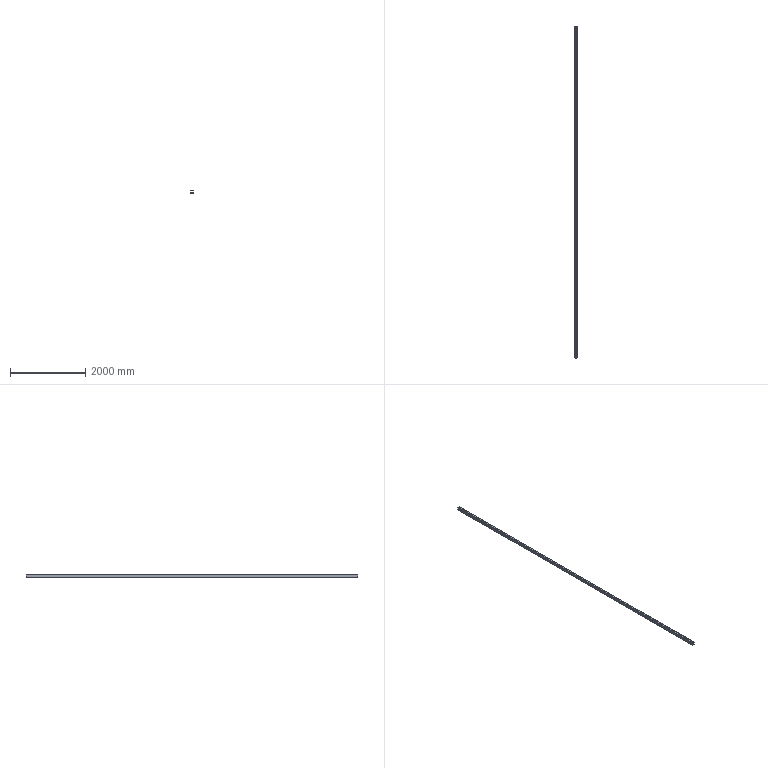Part | SolidWorks | features WeldMemberFeat 1, WeldmentFeature 1 | 1 solid | 18 faces | box 60 x 8850 x 80 mm | volume 10935232 mm3 | plane 10 | cylinder 8 | commonest cylinder face diameters 10 x4 20 x4
STEP:
#1=CARTESIAN_POINT('',(-30.,0.,30.));
#2=VERTEX_POINT('',#1);
#3=CARTESIAN_POINT('',(-20.,0.,40.));
#4=VERTEX_POINT('',#3);
#5=CARTESIAN_POINT('',(-20.,0.,30.));
#6=DIRECTION('',(0.,1.,0.));
#7=DIRECTION('',(0.,0.,1.));
#8=AXIS2_PLACEMENT_3D('',#5,#6,#7);
#9=CIRCLE('',#8,10.);
#10=EDGE_CURVE('',#2,#4,#9,.T.);
#11=ORIENTED_EDGE('',*,*,#10,.T.);
#12=CARTESIAN_POINT('',(-20.,8850.,40.));
#13=VERTEX_POINT('',#12);
#14=CARTESIAN_POINT('',(-20.,8850.,40.));
#15=DIRECTION('',(0.,-1.,0.));
#16=VECTOR('',#15,1000.);
#17=LINE('',#14,#16);
#18=EDGE_CURVE('',#13,#4,#17,.T.);
#19=ORIENTED_EDGE('',*,*,#18,.F.);
#20=CARTESIAN_POINT('',(-30.,8850.,30.));
#21=VERTEX_POINT('',#20);
#22=CARTESIAN_POINT('',(-20.,8850.,30.));
#23=DIRECTION('',(0.,1.,0.));
#24=DIRECTION('',(0.,0.,1.));
#25=AXIS2_PLACEMENT_3D('',#22,#23,#24);
#26=CIRCLE('',#25,10.);
#27=EDGE_CURVE('',#21,#13,#26,.T.);
#28=ORIENTED_EDGE('',*,*,#27,.F.);
#29=CARTESIAN_POINT('',(-30.,8850.,30.));
#30=DIRECTION('',(0.,-1.,0.));
#31=VECTOR('',#30,1000.);
#32=LINE('',#29,#31);
#33=EDGE_CURVE('',#21,#2,#32,.T.);
#34=ORIENTED_EDGE('',*,*,#33,.T.);
#35=EDGE_LOOP('',(#11,#19,#28,#34));
#36=FACE_OUTER_BOUND('',#35,.T.);
#37=CARTESIAN_POINT('',(-20.,8850.,30.));
#38=DIRECTION('',(0.,-1.,0.));
#39=DIRECTION('',(0.,0.,-1.));
#40=AXIS2_PLACEMENT_3D('',#37,#38,#39);
#41=CYLINDRICAL_SURFACE('',#40,10.);
#42=ADVANCED_FACE('',(#36),#41,.T.);
#43=CARTESIAN_POINT('',(20.,0.,40.));
#44=VERTEX_POINT('',#43);
#45=CARTESIAN_POINT('',(-20.,0.,40.));
#46=DIRECTION('',(1.,0.,0.));
#47=VECTOR('',#46,1000.);
#48=LINE('',#45,#47);
#49=EDGE_CURVE('',#4,#44,#48,.T.);
#50=ORIENTED_EDGE('',*,*,#49,.T.);
#51=CARTESIAN_POINT('',(20.,8850.,40.));
#52=VERTEX_POINT('',#51);
#53=CARTESIAN_POINT('',(20.,8850.,40.));
#54=DIRECTION('',(0.,-1.,0.));
#55=VECTOR('',#54,1000.);
#56=LINE('',#53,#55);
#57=EDGE_CURVE('',#52,#44,#56,.T.);
#58=ORIENTED_EDGE('',*,*,#57,.F.);
#59=CARTESIAN_POINT('',(-20.,8850.,40.));
#60=DIRECTION('',(1.,0.,0.));
#61=VECTOR('',#60,1000.);
#62=LINE('',#59,#61);
#63=EDGE_CURVE('',#13,#52,#62,.T.);
#64=ORIENTED_EDGE('',*,*,#63,.F.);
#65=ORIENTED_EDGE('',*,*,#18,.T.);
#66=EDGE_LOOP('',(#50,#58,#64,#65));
#67=FACE_OUTER_BOUND('',#66,.T.);
#68=CARTESIAN_POINT('',(-20.,8850.,40.));
#69=DIRECTION('',(0.,0.,-1.));
#70=DIRECTION('',(-1.,0.,0.));
#71=AXIS2_PLACEMENT_3D('',#68,#69,#70);
#72=PLANE('',#71);
#73=ADVANCED_FACE('',(#67),#72,.F.);
#74=CARTESIAN_POINT('',(30.,0.,30.));
#75=VERTEX_POINT('',#74);
#76=CARTESIAN_POINT('',(20.,0.,30.));
#77=DIRECTION('',(0.,1.,0.));
#78=DIRECTION('',(0.,0.,1.));
#79=AXIS2_PLACEMENT_3D('',#76,#77,#78);
#80=CIRCLE('',#79,10.);
#81=EDGE_CURVE('',#44,#75,#80,.T.);
#82=ORIENTED_EDGE('',*,*,#81,.T.);
#83=CARTESIAN_POINT('',(30.,8850.,30.));
#84=VERTEX_POINT('',#83);
#85=CARTESIAN_POINT('',(30.,8850.,30.));
#86=DIRECTION('',(0.,-1.,0.));
#87=VECTOR('',#86,1000.);
#88=LINE('',#85,#87);
#89=EDGE_CURVE('',#84,#75,#88,.T.);
#90=ORIENTED_EDGE('',*,*,#89,.F.);
#91=CARTESIAN_POINT('',(20.,8850.,30.));
#92=DIRECTION('',(0.,1.,0.));
#93=DIRECTION('',(0.,0.,1.));
#94=AXIS2_PLACEMENT_3D('',#91,#92,#93);
#95=CIRCLE('',#94,10.);
#96=EDGE_CURVE('',#52,#84,#95,.T.);
#97=ORIENTED_EDGE('',*,*,#96,.F.);
#98=ORIENTED_EDGE('',*,*,#57,.T.);
#99=EDGE_LOOP('',(#82,#90,#97,#98));
#100=FACE_OUTER_BOUND('',#99,.T.);
#101=CARTESIAN_POINT('',(20.,8850.,30.));
#102=DIRECTION('',(0.,-1.,0.));
#103=DIRECTION('',(0.,0.,-1.));
#104=AXIS2_PLACEMENT_3D('',#101,#102,#103);
#105=CYLINDRICAL_SURFACE('',#104,10.);
#106=ADVANCED_FACE('',(#100),#105,.T.);
#107=CARTESIAN_POINT('',(30.,0.,-30.));
#108=VERTEX_POINT('',#107);
#109=CARTESIAN_POINT('',(30.,0.,-30.));
#110=DIRECTION('',(0.,0.,-1.));
#111=VECTOR('',#110,1000.);
#112=LINE('',#109,#111);
#113=EDGE_CURVE('',#75,#108,#112,.T.);
#114=ORIENTED_EDGE('',*,*,#113,.T.);
#115=CARTESIAN_POINT('',(30.,8850.,-30.));
#116=VERTEX_POINT('',#115);
#117=CARTESIAN_POINT('',(30.,8850.,-30.));
#118=DIRECTION('',(0.,-1.,0.));
#119=VECTOR('',#118,1000.);
#120=LINE('',#117,#119);
#121=EDGE_CURVE('',#116,#108,#120,.T.);
#122=ORIENTED_EDGE('',*,*,#121,.F.);
#123=CARTESIAN_POINT('',(30.,8850.,-30.));
#124=DIRECTION('',(0.,0.,-1.));
#125=VECTOR('',#124,1000.);
#126=LINE('',#123,#125);
#127=EDGE_CURVE('',#84,#116,#126,.T.);
#128=ORIENTED_EDGE('',*,*,#127,.F.);
#129=ORIENTED_EDGE('',*,*,#89,.T.);
#130=EDGE_LOOP('',(#114,#122,#128,#129));
#131=FACE_OUTER_BOUND('',#130,.T.);
#132=CARTESIAN_POINT('',(30.,8850.,-30.));
#133=DIRECTION('',(-1.,0.,0.));
#134=DIRECTION('',(0.,0.,1.));
#135=AXIS2_PLACEMENT_3D('',#132,#133,#134);
#136=PLANE('',#135);
#137=ADVANCED_FACE('',(#131),#136,.F.);
#138=CARTESIAN_POINT('',(20.,0.,-40.));
#139=VERTEX_POINT('',#138);
#140=CARTESIAN_POINT('',(20.,0.,-30.));
#141=DIRECTION('',(0.,1.,0.));
#142=DIRECTION('',(0.,0.,1.));
#143=AXIS2_PLACEMENT_3D('',#140,#141,#142);
#144=CIRCLE('',#143,10.);
#145=EDGE_CURVE('',#108,#139,#144,.T.);
#146=ORIENTED_EDGE('',*,*,#145,.T.);
#147=CARTESIAN_POINT('',(20.,8850.,-40.));
#148=VERTEX_POINT('',#147);
#149=CARTESIAN_POINT('',(20.,8850.,-40.));
#150=DIRECTION('',(0.,-1.,0.));
#151=VECTOR('',#150,1000.);
#152=LINE('',#149,#151);
#153=EDGE_CURVE('',#148,#139,#152,.T.);
#154=ORIENTED_EDGE('',*,*,#153,.F.);
#155=CARTESIAN_POINT('',(20.,8850.,-30.));
#156=DIRECTION('',(0.,1.,0.));
#157=DIRECTION('',(0.,0.,1.));
#158=AXIS2_PLACEMENT_3D('',#155,#156,#157);
#159=CIRCLE('',#158,10.);
#160=EDGE_CURVE('',#116,#148,#159,.T.);
#161=ORIENTED_EDGE('',*,*,#160,.F.);
#162=ORIENTED_EDGE('',*,*,#121,.T.);
#163=EDGE_LOOP('',(#146,#154,#161,#162));
#164=FACE_OUTER_BOUND('',#163,.T.);
#165=CARTESIAN_POINT('',(20.,8850.,-30.));
#166=DIRECTION('',(0.,-1.,0.));
#167=DIRECTION('',(0.,0.,-1.));
#168=AXIS2_PLACEMENT_3D('',#165,#166,#167);
#169=CYLINDRICAL_SURFACE('',#168,10.);
#170=ADVANCED_FACE('',(#164),#169,.T.);
#171=CARTESIAN_POINT('',(-20.,0.,-40.));
#172=VERTEX_POINT('',#171);
#173=CARTESIAN_POINT('',(20.,0.,-40.));
#174=DIRECTION('',(-1.,0.,0.));
#175=VECTOR('',#174,1000.);
#176=LINE('',#173,#175);
#177=EDGE_CURVE('',#139,#172,#176,.T.);
#178=ORIENTED_EDGE('',*,*,#177,.T.);
#179=CARTESIAN_POINT('',(-20.,8850.,-40.));
#180=VERTEX_POINT('',#179);
#181=CARTESIAN_POINT('',(-20.,8850.,-40.));
#182=DIRECTION('',(0.,-1.,0.));
#183=VECTOR('',#182,1000.);
#184=LINE('',#181,#183);
#185=EDGE_CURVE('',#180,#172,#184,.T.);
#186=ORIENTED_EDGE('',*,*,#185,.F.);
#187=CARTESIAN_POINT('',(20.,8850.,-40.));
#188=DIRECTION('',(-1.,0.,0.));
#189=VECTOR('',#188,1000.);
#190=LINE('',#187,#189);
#191=EDGE_CURVE('',#148,#180,#190,.T.);
#192=ORIENTED_EDGE('',*,*,#191,.F.);
#193=ORIENTED_EDGE('',*,*,#153,.T.);
#194=EDGE_LOOP('',(#178,#186,#192,#193));
#195=FACE_OUTER_BOUND('',#194,.T.);
#196=CARTESIAN_POINT('',(20.,8850.,-40.));
#197=DIRECTION('',(0.,0.,1.));
#198=DIRECTION('',(1.,0.,0.));
#199=AXIS2_PLACEMENT_3D('',#196,#197,#198);
#200=PLANE('',#199);
#201=ADVANCED_FACE('',(#195),#200,.F.);
#202=CARTESIAN_POINT('',(-30.,0.,-30.));
#203=VERTEX_POINT('',#202);
#204=CARTESIAN_POINT('',(-20.,0.,-30.));
#205=DIRECTION('',(0.,1.,0.));
#206=DIRECTION('',(0.,0.,1.));
#207=AXIS2_PLACEMENT_3D('',#204,#205,#206);
#208=CIRCLE('',#207,10.);
#209=EDGE_CURVE('',#172,#203,#208,.T.);
#210=ORIENTED_EDGE('',*,*,#209,.T.);
#211=CARTESIAN_POINT('',(-30.,8850.,-30.));
#212=VERTEX_POINT('',#211);
#213=CARTESIAN_POINT('',(-30.,8850.,-30.));
#214=DIRECTION('',(0.,-1.,0.));
#215=VECTOR('',#214,1000.);
#216=LINE('',#213,#215);
#217=EDGE_CURVE('',#212,#203,#216,.T.);
#218=ORIENTED_EDGE('',*,*,#217,.F.);
#219=CARTESIAN_POINT('',(-20.,8850.,-30.));
#220=DIRECTION('',(0.,1.,0.));
#221=DIRECTION('',(0.,0.,1.));
#222=AXIS2_PLACEMENT_3D('',#219,#220,#221);
#223=CIRCLE('',#222,10.);
#224=EDGE_CURVE('',#180,#212,#223,.T.);
#225=ORIENTED_EDGE('',*,*,#224,.F.);
#226=ORIENTED_EDGE('',*,*,#185,.T.);
#227=EDGE_LOOP('',(#210,#218,#225,#226));
#228=FACE_OUTER_BOUND('',#227,.T.);
#229=CARTESIAN_POINT('',(-20.,8850.,-30.));
#230=DIRECTION('',(0.,-1.,0.));
#231=DIRECTION('',(0.,0.,-1.));
#232=AXIS2_PLACEMENT_3D('',#229,#230,#231);
#233=CYLINDRICAL_SURFACE('',#232,10.);
#234=ADVANCED_FACE('',(#228),#233,.T.);
#235=CARTESIAN_POINT('',(20.,0.,35.));
#236=VERTEX_POINT('',#235);
#237=CARTESIAN_POINT('',(25.,0.,30.));
#238=VERTEX_POINT('',#237);
#239=CARTESIAN_POINT('',(20.,0.,30.));
#240=DIRECTION('',(0.,1.,0.));
#241=DIRECTION('',(0.,0.,1.));
#242=AXIS2_PLACEMENT_3D('',#239,#240,#241);
#243=CIRCLE('',#242,5.);
#244=EDGE_CURVE('',#236,#238,#243,.T.);
#245=ORIENTED_EDGE('',*,*,#244,.F.);
#246=CARTESIAN_POINT('',(20.,8850.,35.));
#247=VERTEX_POINT('',#246);
#248=CARTESIAN_POINT('',(20.,8850.,35.));
#249=DIRECTION('',(0.,-1.,0.));
#250=VECTOR('',#249,1000.);
#251=LINE('',#248,#250);
#252=EDGE_CURVE('',#247,#236,#251,.T.);
#253=ORIENTED_EDGE('',*,*,#252,.F.);
#254=CARTESIAN_POINT('',(25.,8850.,30.));
#255=VERTEX_POINT('',#254);
#256=CARTESIAN_POINT('',(20.,8850.,30.));
#257=DIRECTION('',(0.,1.,0.));
#258=DIRECTION('',(0.,0.,1.));
#259=AXIS2_PLACEMENT_3D('',#256,#257,#258);
#260=CIRCLE('',#259,5.);
#261=EDGE_CURVE('',#247,#255,#260,.T.);
#262=ORIENTED_EDGE('',*,*,#261,.T.);
#263=CARTESIAN_POINT('',(25.,8850.,30.));
#264=DIRECTION('',(0.,-1.,0.));
#265=VECTOR('',#264,1000.);
#266=LINE('',#263,#265);
#267=EDGE_CURVE('',#255,#238,#266,.T.);
#268=ORIENTED_EDGE('',*,*,#267,.T.);
#269=EDGE_LOOP('',(#245,#253,#262,#268));
#270=FACE_OUTER_BOUND('',#269,.T.);
#271=CARTESIAN_POINT('',(20.,8850.,30.));
#272=DIRECTION('',(0.,-1.,0.));
#273=DIRECTION('',(0.,0.,-1.));
#274=AXIS2_PLACEMENT_3D('',#271,#272,#273);
#275=CYLINDRICAL_SURFACE('',#274,5.);
#276=ADVANCED_FACE('',(#270),#275,.F.);
#277=CARTESIAN_POINT('',(-20.,0.,35.));
#278=VERTEX_POINT('',#277);
#279=CARTESIAN_POINT('',(-20.,0.,35.));
#280=DIRECTION('',(1.,0.,0.));
#281=VECTOR('',#280,1000.);
#282=LINE('',#279,#281);
#283=EDGE_CURVE('',#278,#236,#282,.T.);
#284=ORIENTED_EDGE('',*,*,#283,.F.);
#285=CARTESIAN_POINT('',(-20.,8850.,35.));
#286=VERTEX_POINT('',#285);
#287=CARTESIAN_POINT('',(-20.,8850.,35.));
#288=DIRECTION('',(0.,-1.,0.));
#289=VECTOR('',#288,1000.);
#290=LINE('',#287,#289);
#291=EDGE_CURVE('',#286,#278,#290,.T.);
#292=ORIENTED_EDGE('',*,*,#291,.F.);
#293=CARTESIAN_POINT('',(-20.,8850.,35.));
#294=DIRECTION('',(1.,0.,0.));
#295=VECTOR('',#294,1000.);
#296=LINE('',#293,#295);
#297=EDGE_CURVE('',#286,#247,#296,.T.);
#298=ORIENTED_EDGE('',*,*,#297,.T.);
#299=ORIENTED_EDGE('',*,*,#252,.T.);
#300=EDGE_LOOP('',(#284,#292,#298,#299));
#301=FACE_OUTER_BOUND('',#300,.T.);
#302=CARTESIAN_POINT('',(-20.,8850.,35.));
#303=DIRECTION('',(0.,0.,-1.));
#304=DIRECTION('',(-1.,0.,0.));
#305=AXIS2_PLACEMENT_3D('',#302,#303,#304);
#306=PLANE('',#305);
#307=ADVANCED_FACE('',(#301),#306,.T.);
#308=CARTESIAN_POINT('',(-25.,0.,30.));
#309=VERTEX_POINT('',#308);
#310=CARTESIAN_POINT('',(-20.,0.,30.));
#311=DIRECTION('',(0.,1.,0.));
#312=DIRECTION('',(0.,0.,1.));
#313=AXIS2_PLACEMENT_3D('',#310,#311,#312);
#314=CIRCLE('',#313,5.);
#315=EDGE_CURVE('',#309,#278,#314,.T.);
#316=ORIENTED_EDGE('',*,*,#315,.F.);
#317=CARTESIAN_POINT('',(-25.,8850.,30.));
#318=VERTEX_POINT('',#317);
#319=CARTESIAN_POINT('',(-25.,8850.,30.));
#320=DIRECTION('',(0.,-1.,0.));
#321=VECTOR('',#320,1000.);
#322=LINE('',#319,#321);
#323=EDGE_CURVE('',#318,#309,#322,.T.);
#324=ORIENTED_EDGE('',*,*,#323,.F.);
#325=CARTESIAN_POINT('',(-20.,8850.,30.));
#326=DIRECTION('',(0.,1.,0.));
#327=DIRECTION('',(0.,0.,1.));
#328=AXIS2_PLACEMENT_3D('',#325,#326,#327);
#329=CIRCLE('',#328,5.);
#330=EDGE_CURVE('',#318,#286,#329,.T.);
#331=ORIENTED_EDGE('',*,*,#330,.T.);
#332=ORIENTED_EDGE('',*,*,#291,.T.);
#333=EDGE_LOOP('',(#316,#324,#331,#332));
#334=FACE_OUTER_BOUND('',#333,.T.);
#335=CARTESIAN_POINT('',(-20.,8850.,30.));
#336=DIRECTION('',(0.,-1.,0.));
#337=DIRECTION('',(0.,0.,-1.));
#338=AXIS2_PLACEMENT_3D('',#335,#336,#337);
#339=CYLINDRICAL_SURFACE('',#338,5.);
#340=ADVANCED_FACE('',(#334),#339,.F.);
#341=CARTESIAN_POINT('',(-25.,0.,-30.));
#342=VERTEX_POINT('',#341);
#343=CARTESIAN_POINT('',(-25.,0.,30.));
#344=DIRECTION('',(0.,0.,1.));
#345=VECTOR('',#344,1000.);
#346=LINE('',#343,#345);
#347=EDGE_CURVE('',#342,#309,#346,.T.);
#348=ORIENTED_EDGE('',*,*,#347,.F.);
#349=CARTESIAN_POINT('',(-25.,8850.,-30.));
#350=VERTEX_POINT('',#349);
#351=CARTESIAN_POINT('',(-25.,8850.,-30.));
#352=DIRECTION('',(0.,-1.,0.));
#353=VECTOR('',#352,1000.);
#354=LINE('',#351,#353);
#355=EDGE_CURVE('',#350,#342,#354,.T.);
#356=ORIENTED_EDGE('',*,*,#355,.F.);
#357=CARTESIAN_POINT('',(-25.,8850.,30.));
#358=DIRECTION('',(0.,0.,1.));
#359=VECTOR('',#358,1000.);
#360=LINE('',#357,#359);
#361=EDGE_CURVE('',#350,#318,#360,.T.);
#362=ORIENTED_EDGE('',*,*,#361,.T.);
#363=ORIENTED_EDGE('',*,*,#323,.T.);
#364=EDGE_LOOP('',(#348,#356,#362,#363));
#365=FACE_OUTER_BOUND('',#364,.T.);
#366=CARTESIAN_POINT('',(-25.,8850.,30.));
#367=DIRECTION('',(1.,0.,0.));
#368=DIRECTION('',(0.,0.,-1.));
#369=AXIS2_PLACEMENT_3D('',#366,#367,#368);
#370=PLANE('',#369);
#371=ADVANCED_FACE('',(#365),#370,.T.);
#372=CARTESIAN_POINT('',(-20.,0.,-35.));
#373=VERTEX_POINT('',#372);
#374=CARTESIAN_POINT('',(-20.,0.,-30.));
#375=DIRECTION('',(0.,1.,0.));
#376=DIRECTION('',(0.,0.,1.));
#377=AXIS2_PLACEMENT_3D('',#374,#375,#376);
#378=CIRCLE('',#377,5.);
#379=EDGE_CURVE('',#373,#342,#378,.T.);
#380=ORIENTED_EDGE('',*,*,#379,.F.);
#381=CARTESIAN_POINT('',(-20.,8850.,-35.));
#382=VERTEX_POINT('',#381);
#383=CARTESIAN_POINT('',(-20.,8850.,-35.));
#384=DIRECTION('',(0.,-1.,0.));
#385=VECTOR('',#384,1000.);
#386=LINE('',#383,#385);
#387=EDGE_CURVE('',#382,#373,#386,.T.);
#388=ORIENTED_EDGE('',*,*,#387,.F.);
#389=CARTESIAN_POINT('',(-20.,8850.,-30.));
#390=DIRECTION('',(0.,1.,0.));
#391=DIRECTION('',(0.,0.,1.));
#392=AXIS2_PLACEMENT_3D('',#389,#390,#391);
#393=CIRCLE('',#392,5.);
#394=EDGE_CURVE('',#382,#350,#393,.T.);
#395=ORIENTED_EDGE('',*,*,#394,.T.);
#396=ORIENTED_EDGE('',*,*,#355,.T.);
#397=EDGE_LOOP('',(#380,#388,#395,#396));
#398=FACE_OUTER_BOUND('',#397,.T.);
#399=CARTESIAN_POINT('',(-20.,8850.,-30.));
#400=DIRECTION('',(0.,-1.,0.));
#401=DIRECTION('',(0.,0.,-1.));
#402=AXIS2_PLACEMENT_3D('',#399,#400,#401);
#403=CYLINDRICAL_SURFACE('',#402,5.);
#404=ADVANCED_FACE('',(#398),#403,.F.);
#405=CARTESIAN_POINT('',(20.,0.,-35.));
#406=VERTEX_POINT('',#405);
#407=CARTESIAN_POINT('',(20.,0.,-35.));
#408=DIRECTION('',(-1.,0.,0.));
#409=VECTOR('',#408,1000.);
#410=LINE('',#407,#409);
#411=EDGE_CURVE('',#406,#373,#410,.T.);
#412=ORIENTED_EDGE('',*,*,#411,.F.);
#413=CARTESIAN_POINT('',(20.,8850.,-35.));
#414=VERTEX_POINT('',#413);
#415=CARTESIAN_POINT('',(20.,8850.,-35.));
#416=DIRECTION('',(0.,-1.,0.));
#417=VECTOR('',#416,1000.);
#418=LINE('',#415,#417);
#419=EDGE_CURVE('',#414,#406,#418,.T.);
#420=ORIENTED_EDGE('',*,*,#419,.F.);
#421=CARTESIAN_POINT('',(20.,8850.,-35.));
#422=DIRECTION('',(-1.,0.,0.));
#423=VECTOR('',#422,1000.);
#424=LINE('',#421,#423);
#425=EDGE_CURVE('',#414,#382,#424,.T.);
#426=ORIENTED_EDGE('',*,*,#425,.T.);
#427=ORIENTED_EDGE('',*,*,#387,.T.);
#428=EDGE_LOOP('',(#412,#420,#426,#427));
#429=FACE_OUTER_BOUND('',#428,.T.);
#430=CARTESIAN_POINT('',(20.,8850.,-35.));
#431=DIRECTION('',(0.,0.,1.));
#432=DIRECTION('',(1.,0.,0.));
#433=AXIS2_PLACEMENT_3D('',#430,#431,#432);
#434=PLANE('',#433);
#435=ADVANCED_FACE('',(#429),#434,.T.);
#436=CARTESIAN_POINT('',(25.,0.,-30.));
#437=VERTEX_POINT('',#436);
#438=CARTESIAN_POINT('',(20.,0.,-30.));
#439=DIRECTION('',(0.,1.,0.));
#440=DIRECTION('',(0.,0.,1.));
#441=AXIS2_PLACEMENT_3D('',#438,#439,#440);
#442=CIRCLE('',#441,5.);
#443=EDGE_CURVE('',#437,#406,#442,.T.);
#444=ORIENTED_EDGE('',*,*,#443,.F.);
#445=CARTESIAN_POINT('',(25.,8850.,-30.));
#446=VERTEX_POINT('',#445);
#447=CARTESIAN_POINT('',(25.,8850.,-30.));
#448=DIRECTION('',(0.,-1.,0.));
#449=VECTOR('',#448,1000.);
#450=LINE('',#447,#449);
#451=EDGE_CURVE('',#446,#437,#450,.T.);
#452=ORIENTED_EDGE('',*,*,#451,.F.);
#453=CARTESIAN_POINT('',(20.,8850.,-30.));
#454=DIRECTION('',(0.,1.,0.));
#455=DIRECTION('',(0.,0.,1.));
#456=AXIS2_PLACEMENT_3D('',#453,#454,#455);
#457=CIRCLE('',#456,5.);
#458=EDGE_CURVE('',#446,#414,#457,.T.);
#459=ORIENTED_EDGE('',*,*,#458,.T.);
#460=ORIENTED_EDGE('',*,*,#419,.T.);
#461=EDGE_LOOP('',(#444,#452,#459,#460));
#462=FACE_OUTER_BOUND('',#461,.T.);
#463=CARTESIAN_POINT('',(20.,8850.,-30.));
#464=DIRECTION('',(0.,-1.,0.));
#465=DIRECTION('',(0.,0.,-1.));
#466=AXIS2_PLACEMENT_3D('',#463,#464,#465);
#467=CYLINDRICAL_SURFACE('',#466,5.);
#468=ADVANCED_FACE('',(#462),#467,.F.);
#469=CARTESIAN_POINT('',(25.,0.,-30.));
#470=DIRECTION('',(0.,0.,-1.));
#471=VECTOR('',#470,1000.);
#472=LINE('',#469,#471);
#473=EDGE_CURVE('',#238,#437,#472,.T.);
#474=ORIENTED_EDGE('',*,*,#473,.F.);
#475=ORIENTED_EDGE('',*,*,#267,.F.);
#476=CARTESIAN_POINT('',(25.,8850.,-30.));
#477=DIRECTION('',(0.,0.,-1.));
#478=VECTOR('',#477,1000.);
#479=LINE('',#476,#478);
#480=EDGE_CURVE('',#255,#446,#479,.T.);
#481=ORIENTED_EDGE('',*,*,#480,.T.);
#482=ORIENTED_EDGE('',*,*,#451,.T.);
#483=EDGE_LOOP('',(#474,#475,#481,#482));
#484=FACE_OUTER_BOUND('',#483,.T.);
#485=CARTESIAN_POINT('',(25.,8850.,-30.));
#486=DIRECTION('',(-1.,0.,0.));
#487=DIRECTION('',(0.,0.,1.));
#488=AXIS2_PLACEMENT_3D('',#485,#486,#487);
#489=PLANE('',#488);
#490=ADVANCED_FACE('',(#484),#489,.T.);
#491=CARTESIAN_POINT('',(-30.,0.,30.));
#492=DIRECTION('',(0.,0.,1.));
#493=VECTOR('',#492,1000.);
#494=LINE('',#491,#493);
#495=EDGE_CURVE('',#203,#2,#494,.T.);
#496=ORIENTED_EDGE('',*,*,#495,.T.);
#497=ORIENTED_EDGE('',*,*,#33,.F.);
#498=CARTESIAN_POINT('',(-30.,8850.,30.));
#499=DIRECTION('',(0.,0.,1.));
#500=VECTOR('',#499,1000.);
#501=LINE('',#498,#500);
#502=EDGE_CURVE('',#212,#21,#501,.T.);
#503=ORIENTED_EDGE('',*,*,#502,.F.);
#504=ORIENTED_EDGE('',*,*,#217,.T.);
#505=EDGE_LOOP('',(#496,#497,#503,#504));
#506=FACE_OUTER_BOUND('',#505,.T.);
#507=CARTESIAN_POINT('',(-30.,8850.,30.));
#508=DIRECTION('',(1.,0.,0.));
#509=DIRECTION('',(0.,0.,-1.));
#510=AXIS2_PLACEMENT_3D('',#507,#508,#509);
#511=PLANE('',#510);
#512=ADVANCED_FACE('',(#506),#511,.F.);
#513=ORIENTED_EDGE('',*,*,#261,.F.);
#514=ORIENTED_EDGE('',*,*,#297,.F.);
#515=ORIENTED_EDGE('',*,*,#330,.F.);
#516=ORIENTED_EDGE('',*,*,#361,.F.);
#517=ORIENTED_EDGE('',*,*,#394,.F.);
#518=ORIENTED_EDGE('',*,*,#425,.F.);
#519=ORIENTED_EDGE('',*,*,#458,.F.);
#520=ORIENTED_EDGE('',*,*,#480,.F.);
#521=EDGE_LOOP('',(#513,#514,#515,#516,#517,#518,#519,#520));
#522=FACE_BOUND('',#521,.T.);
#523=ORIENTED_EDGE('',*,*,#27,.T.);
#524=ORIENTED_EDGE('',*,*,#63,.T.);
#525=ORIENTED_EDGE('',*,*,#96,.T.);
#526=ORIENTED_EDGE('',*,*,#127,.T.);
#527=ORIENTED_EDGE('',*,*,#160,.T.);
#528=ORIENTED_EDGE('',*,*,#191,.T.);
#529=ORIENTED_EDGE('',*,*,#224,.T.);
#530=ORIENTED_EDGE('',*,*,#502,.T.);
#531=EDGE_LOOP('',(#523,#524,#525,#526,#527,#528,#529,#530));
#532=FACE_OUTER_BOUND('',#531,.T.);
#533=CARTESIAN_POINT('',(-20.,8850.,30.));
#534=DIRECTION('',(0.,1.,0.));
#535=DIRECTION('',(0.,0.,1.));
#536=AXIS2_PLACEMENT_3D('',#533,#534,#535);
#537=PLANE('',#536);
#538=ADVANCED_FACE('',(#522,#532),#537,.T.);
#539=ORIENTED_EDGE('',*,*,#244,.T.);
#540=ORIENTED_EDGE('',*,*,#473,.T.);
#541=ORIENTED_EDGE('',*,*,#443,.T.);
#542=ORIENTED_EDGE('',*,*,#411,.T.);
#543=ORIENTED_EDGE('',*,*,#379,.T.);
#544=ORIENTED_EDGE('',*,*,#347,.T.);
#545=ORIENTED_EDGE('',*,*,#315,.T.);
#546=ORIENTED_EDGE('',*,*,#283,.T.);
#547=EDGE_LOOP('',(#539,#540,#541,#542,#543,#544,#545,#546));
#548=FACE_BOUND('',#547,.T.);
#549=ORIENTED_EDGE('',*,*,#10,.F.);
#550=ORIENTED_EDGE('',*,*,#495,.F.);
#551=ORIENTED_EDGE('',*,*,#209,.F.);
#552=ORIENTED_EDGE('',*,*,#177,.F.);
#553=ORIENTED_EDGE('',*,*,#145,.F.);
#554=ORIENTED_EDGE('',*,*,#113,.F.);
#555=ORIENTED_EDGE('',*,*,#81,.F.);
#556=ORIENTED_EDGE('',*,*,#49,.F.);
#557=EDGE_LOOP('',(#549,#550,#551,#552,#553,#554,#555,#556));
#558=FACE_OUTER_BOUND('',#557,.T.);
#559=CARTESIAN_POINT('',(-20.,0.,30.));
#560=DIRECTION('',(0.,1.,0.));
#561=DIRECTION('',(0.,0.,1.));
#562=AXIS2_PLACEMENT_3D('',#559,#560,#561);
#563=PLANE('',#562);
#564=ADVANCED_FACE('',(#548,#558),#563,.F.);
#565=CLOSED_SHELL('',(#42,#73,#106,#137,#170,#201,#234,#276,#307,#340,#371,#404,#435,#468,#490,#512,#538,#564));
#566=MANIFOLD_SOLID_BREP('',#565);
#567=CARTESIAN_POINT('',(0.,0.,0.));
#568=DIRECTION('',(0.,0.,1.));
#569=DIRECTION('',(1.,0.,0.));
#570=AXIS2_PLACEMENT_3D('',#567,#568,#569);
#571=(LENGTH_UNIT()NAMED_UNIT(*)SI_UNIT(.MILLI.,.METRE.));
#572=UNCERTAINTY_MEASURE_WITH_UNIT(LENGTH_MEASURE(0.00001),#571,'','');
#573=(NAMED_UNIT(*)PLANE_ANGLE_UNIT()SI_UNIT($,.RADIAN.));
#574=(NAMED_UNIT(*)SI_UNIT($,.STERADIAN.)SOLID_ANGLE_UNIT());
#575=(GEOMETRIC_REPRESENTATION_CONTEXT(3)GLOBAL_UNCERTAINTY_ASSIGNED_CONTEXT((#572))GLOBAL_UNIT_ASSIGNED_CONTEXT((#571,#573,#574))REPRESENTATION_CONTEXT('',''));
#576=ADVANCED_BREP_SHAPE_REPRESENTATION('',(#566,#570),#575);